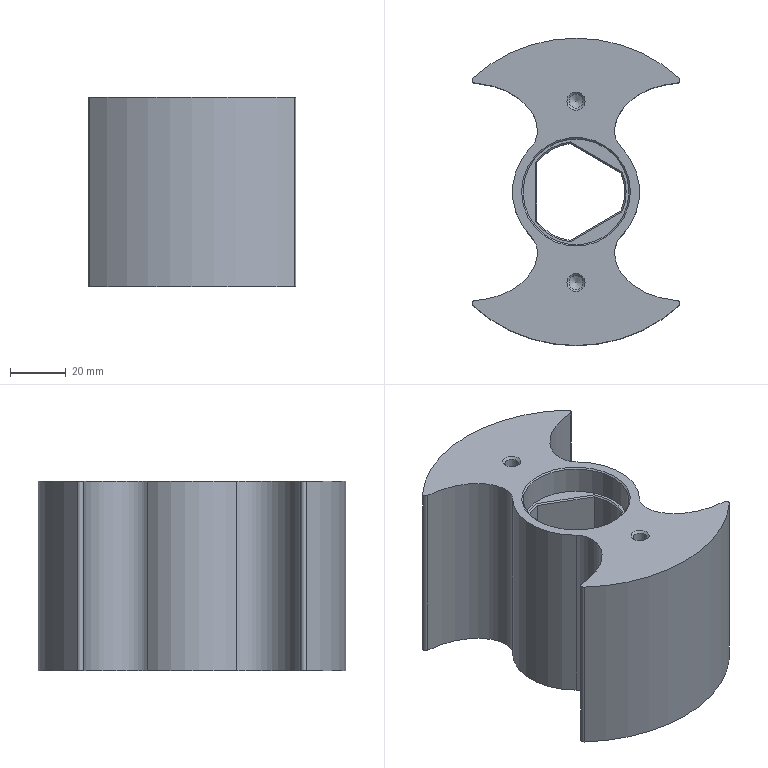NC program | NX | posted with a generic post | part box 74.46 x 110.159 x 68 mm
Lines 28 to 1004 of 5030:
(ZLEVEL_PROFILE_COPY_1 , TOOL : D12)
N48 M6
N50 G54
N52 G17 G0 G90 X7.103 Y-3.397 S3000 M3
N54 G43 Z30. H12
N56 Z-2.
N58 G94 G1 X10.893 Y3.167 Z-2.198 F1000.
N60 X10.665 Y3.958 Z-2.22
N62 X9.854 Y5.689 Z-2.27
N64 X8.765 Y7.258 Z-2.32
N66 X8.195 Y7.853 Z-2.342
N68 X8.017 Y7.85 Z-2.346
N70 X-8.183 Z-2.771
N72 X-8.282 Y7.761 Z-2.774
N74 X-8.844 Y7.163 Z-2.796
N76 X-9.887 Y5.632 Z-2.844
N78 X-10.665 Y3.951 Z-2.893
N80 X-10.89 Y3.162 Z-2.914
N82 X-2.794 Y-10.861 Z-3.338
N84 X-2.704 Y-11.023 Z-3.343
N86 X-1.898 Y-11.219 Z-3.365
N88 X-0.048 Y-11.377 Z-3.413
N90 X1.802 Y-11.235 Z-3.462
N92 X2.61 Y-11.046 Z-3.484
N94 X2.707 Y-11.012 Z-3.486
N96 X10.893 Y3.167 Z-3.915
N98 X10.665 Y3.958 Z-3.937
N100 X9.854 Y5.689 Z-3.987
N102 X8.765 Y7.258 Z-4.037
N104 X8.195 Y7.853 Z-4.058
N106 X8.017 Y7.85 Z-4.063
N108 X-8.183 Z-4.487
N110 X-8.282 Y7.761 Z-4.49
N112 X-8.844 Y7.163 Z-4.512
N114 X-9.887 Y5.632 Z-4.56
N116 X-10.665 Y3.951 Z-4.609
N118 X-10.89 Y3.162 Z-4.63
N120 X-2.794 Y-10.861 Z-5.054
N122 X-2.704 Y-11.023 Z-5.059
N124 X-1.898 Y-11.219 Z-5.081
N126 X-0.048 Y-11.377 Z-5.13
N128 X1.802 Y-11.235 Z-5.178
N130 X2.61 Y-11.046 Z-5.2
N132 X2.707 Y-11.012 F1800.
N134 X10.893 Y3.167
N136 G3 X8.195 Y7.853 R11.295
N138 G1 X8.017 Y7.85
N140 X-8.183
N142 X-8.282 Y7.761
N144 G3 X-10.89 Y3.162 R11.205
N146 G1 X-2.794 Y-10.861
N148 X-2.704 Y-11.023
N150 G3 X2.61 Y-11.046 R11.457
N152 G1 X2.691 Y-11.014 Z-5.202
N154 X3.065 Y-10.392 Z-5.214
N156 X8.385 Y-1.178 Z-5.4
N158 X10.893 Y3.167
N160 G3 X8.195 Y7.853 R11.295
N162 G1 X8.017 Y7.85
N164 X-8.183
N166 X-8.282 Y7.761
N168 G3 X-10.89 Y3.162 R11.205
N170 G1 X-2.794 Y-10.861
N172 X-2.704 Y-11.023
N174 G3 X2.61 Y-11.046 R11.457
N176 G1 X2.691 Y-11.014 Z-5.402
N178 X3.065 Y-10.392 Z-5.414
N180 X8.385 Y-1.178 Z-5.6
N182 X10.9 Y3.179
N184 X10.855 Y3.316
N186 G3 X8.195 Y7.853 R11.35
N188 G1 X8.017 Y7.85
N190 X-8.193
N192 X-8.282 Y7.761
N194 G3 X-10.859 Y3.303 R11.35
N196 G1 X-10.9 Y3.179
N198 X-2.794 Y-10.861
N200 X-2.704 Y-11.023
N202 G3 X2.61 Y-11.046 R11.35
N204 G1 X2.691 Y-11.014 Z-5.602
N206 X3.063 Y-10.394 Z-5.614
N208 X8.383 Y-1.18 Z-5.8
N210 X10.9 Y3.179
N212 X10.855 Y3.316
N214 G3 X8.195 Y7.853 R11.35
N216 G1 X8.017 Y7.85
N218 X-8.193
N220 X-8.282 Y7.761
N222 G3 X-10.859 Y3.303 R11.35
N224 G1 X-10.9 Y3.179
N226 X-2.794 Y-10.861
N228 X-2.704 Y-11.023
N230 G3 X2.61 Y-11.046 R11.35
N232 G1 X2.696 Y-11.013 Z-5.802
N234 X3.063 Y-10.394 Z-5.814
N236 X8.383 Y-1.18 Z-6.
N238 X10.9 Y3.179
N240 X10.855 Y3.316
N242 G3 X8.195 Y7.853 R11.35
N244 G1 X8.017 Y7.85
N246 X-8.193
N248 X-8.282 Y7.761
N250 G3 X-10.859 Y3.303 R11.35
N252 G1 X-10.9 Y3.179
N254 X-2.794 Y-10.861
N256 X-2.704 Y-11.023
N258 G3 X2.61 Y-11.046 R11.35
N260 G1 X2.696 Y-11.013 Z-6.002
N262 X3.063 Y-10.394 Z-6.014
N264 X8.383 Y-1.18 Z-6.2
N266 X10.9 Y3.179
N268 X10.855 Y3.316
N270 G3 X8.195 Y7.853 R11.35
N272 G1 X8.017 Y7.85
N274 X-8.193
N276 X-8.282 Y7.761
N278 G3 X-10.859 Y3.303 R11.35
N280 G1 X-10.9 Y3.179
N282 X-2.794 Y-10.861
N284 X-2.704 Y-11.023
N286 G3 X2.61 Y-11.046 R11.35
N288 G1 X2.696 Y-11.013 Z-6.202
N290 X3.063 Y-10.394 Z-6.214
N292 X8.383 Y-1.18 Z-6.4
N294 X10.9 Y3.179
N296 X10.855 Y3.316
N298 G3 X8.195 Y7.853 R11.35
N300 G1 X8.017 Y7.85
N302 X-8.193
N304 X-8.282 Y7.761
N306 G3 X-10.859 Y3.303 R11.35
N308 G1 X-10.9 Y3.179
N310 X-2.794 Y-10.861
N312 X-2.704 Y-11.023
N314 G3 X2.61 Y-11.046 R11.35
N316 G1 X2.696 Y-11.013 Z-6.402
N318 X3.063 Y-10.394 Z-6.414
N320 X8.383 Y-1.18 Z-6.6
N322 X10.9 Y3.179
N324 X10.855 Y3.316
N326 G3 X8.195 Y7.853 R11.35
N328 G1 X8.017 Y7.85
N330 X-8.193
N332 X-8.282 Y7.761
N334 G3 X-10.859 Y3.303 R11.35
N336 G1 X-10.9 Y3.179
N338 X-2.794 Y-10.861
N340 X-2.704 Y-11.023
N342 G3 X2.61 Y-11.046 R11.35
N344 G1 X2.696 Y-11.013 Z-6.602
N346 X3.063 Y-10.394 Z-6.614
N348 X8.383 Y-1.18 Z-6.8
N350 X10.9 Y3.179
N352 X10.855 Y3.316
N354 G3 X8.195 Y7.853 R11.35
N356 G1 X8.017 Y7.85
N358 X-8.193
N360 X-8.282 Y7.761
N362 G3 X-10.859 Y3.303 R11.35
N364 G1 X-10.9 Y3.179
N366 X-2.794 Y-10.861
N368 X-2.704 Y-11.023
N370 G3 X2.61 Y-11.046 R11.35
N372 G1 X2.696 Y-11.013 Z-6.802
N374 X3.063 Y-10.394 Z-6.814
N376 X8.383 Y-1.18 Z-7.
N378 X10.9 Y3.179
N380 X10.855 Y3.316
N382 G3 X8.195 Y7.853 R11.35
N384 G1 X8.017 Y7.85
N386 X-8.193
N388 X-8.282 Y7.761
N390 G3 X-10.859 Y3.303 R11.35
N392 G1 X-10.9 Y3.179
N394 X-2.794 Y-10.861
N396 X-2.704 Y-11.023
N398 G3 X2.61 Y-11.046 R11.35
N400 G1 X2.696 Y-11.013 Z-7.002
N402 X3.063 Y-10.394 Z-7.014
N404 X8.383 Y-1.18 Z-7.2
N406 X10.9 Y3.179
N408 X10.855 Y3.316
N410 G3 X8.195 Y7.853 R11.35
N412 G1 X8.017 Y7.85
N414 X-8.193
N416 X-8.282 Y7.761
N418 G3 X-10.859 Y3.303 R11.35
N420 G1 X-10.9 Y3.179
N422 X-2.794 Y-10.861
N424 X-2.704 Y-11.023
N426 G3 X2.61 Y-11.046 R11.35
N428 G1 X2.696 Y-11.013 Z-7.202
N430 X3.063 Y-10.394 Z-7.214
N432 X8.383 Y-1.18 Z-7.4
N434 X10.9 Y3.179
N436 X10.855 Y3.316
N438 G3 X8.195 Y7.853 R11.35
N440 G1 X8.017 Y7.85
N442 X-8.193
N444 X-8.282 Y7.761
N446 G3 X-10.859 Y3.303 R11.35
N448 G1 X-10.9 Y3.179
N450 X-2.794 Y-10.861
N452 X-2.704 Y-11.023
N454 G3 X2.61 Y-11.046 R11.35
N456 G1 X2.696 Y-11.013 Z-7.402
N458 X3.063 Y-10.394 Z-7.414
N460 X8.383 Y-1.18 Z-7.6
N462 X10.9 Y3.179
N464 X10.855 Y3.316
N466 G3 X8.195 Y7.853 R11.35
N468 G1 X8.017 Y7.85
N470 X-8.193
N472 X-8.282 Y7.761
N474 G3 X-10.859 Y3.303 R11.35
N476 G1 X-10.9 Y3.179
N478 X-2.794 Y-10.861
N480 X-2.704 Y-11.023
N482 G3 X2.61 Y-11.046 R11.35
N484 G1 X2.696 Y-11.013 Z-7.602
N486 X3.063 Y-10.394 Z-7.614
N488 X8.383 Y-1.18 Z-7.8
N490 X10.9 Y3.179
N492 X10.855 Y3.316
N494 G3 X8.195 Y7.853 R11.35
N496 G1 X8.017 Y7.85
N498 X-8.193
N500 X-8.282 Y7.761
N502 G3 X-10.859 Y3.303 R11.35
N504 G1 X-10.9 Y3.179
N506 X-2.794 Y-10.861
N508 X-2.704 Y-11.023
N510 G3 X2.61 Y-11.046 R11.35
N512 G1 X2.696 Y-11.013 Z-7.802
N514 X3.063 Y-10.394 Z-7.814
N516 X8.383 Y-1.18 Z-8.
N518 X10.9 Y3.179
N520 X10.855 Y3.316
N522 G3 X8.195 Y7.853 R11.35
N524 G1 X8.017 Y7.85
N526 X-8.193
N528 X-8.282 Y7.761
N530 G3 X-10.859 Y3.303 R11.35
N532 G1 X-10.9 Y3.179
N534 X-2.794 Y-10.861
N536 X-2.704 Y-11.023
N538 G3 X2.61 Y-11.046 R11.35
N540 G1 X2.696 Y-11.013 Z-8.002
N542 X3.063 Y-10.394 Z-8.014
N544 X8.383 Y-1.18 Z-8.2
N546 X10.9 Y3.179
N548 X10.855 Y3.316
N550 G3 X8.195 Y7.853 R11.35
N552 G1 X8.017 Y7.85
N554 X-8.193
N556 X-8.282 Y7.761
N558 G3 X-10.859 Y3.303 R11.35
N560 G1 X-10.9 Y3.179
N562 X-2.794 Y-10.861
N564 X-2.704 Y-11.023
N566 G3 X2.61 Y-11.046 R11.35
N568 G1 X2.696 Y-11.013 Z-8.202
N570 X3.063 Y-10.394 Z-8.214
N572 X8.383 Y-1.18 Z-8.4
N574 X10.9 Y3.179
N576 X10.855 Y3.316
N578 G3 X8.195 Y7.853 R11.35
N580 G1 X8.017 Y7.85
N582 X-8.193
N584 X-8.282 Y7.761
N586 G3 X-10.859 Y3.303 R11.35
N588 G1 X-10.9 Y3.179
N590 X-2.794 Y-10.861
N592 X-2.704 Y-11.023
N594 G3 X2.61 Y-11.046 R11.35
N596 G1 X2.696 Y-11.013 Z-8.402
N598 X3.063 Y-10.394 Z-8.414
N600 X8.383 Y-1.18 Z-8.6
N602 X10.9 Y3.179
N604 X10.855 Y3.316
N606 G3 X8.195 Y7.853 R11.35
N608 G1 X8.017 Y7.85
N610 X-8.193
N612 X-8.282 Y7.761
N614 G3 X-10.859 Y3.303 R11.35
N616 G1 X-10.9 Y3.179
N618 X-2.794 Y-10.861
N620 X-2.704 Y-11.023
N622 G3 X2.61 Y-11.046 R11.35
N624 G1 X2.696 Y-11.013 Z-8.602
N626 X3.063 Y-10.394 Z-8.614
N628 X8.383 Y-1.18 Z-8.8
N630 X10.9 Y3.179
N632 X10.855 Y3.316
N634 G3 X8.195 Y7.853 R11.35
N636 G1 X8.017 Y7.85
N638 X-8.193
N640 X-8.282 Y7.761
N642 G3 X-10.859 Y3.303 R11.35
N644 G1 X-10.9 Y3.179
N646 X-2.794 Y-10.861
N648 X-2.704 Y-11.023
N650 G3 X2.61 Y-11.046 R11.35
N652 G1 X2.696 Y-11.013 Z-8.802
N654 X3.063 Y-10.394 Z-8.814
N656 X8.383 Y-1.18 Z-9.
N658 X10.9 Y3.179
N660 X10.855 Y3.316
N662 G3 X8.195 Y7.853 R11.35
N664 G1 X8.017 Y7.85
N666 X-8.193
N668 X-8.282 Y7.761
N670 G3 X-10.859 Y3.303 R11.35
N672 G1 X-10.9 Y3.179
N674 X-2.794 Y-10.861
N676 X-2.704 Y-11.023
N678 G3 X2.61 Y-11.046 R11.35
N680 G1 X2.696 Y-11.013 Z-9.002
N682 X3.063 Y-10.394 Z-9.014
N684 X8.383 Y-1.18 Z-9.2
N686 X10.9 Y3.179
N688 X10.855 Y3.316
N690 G3 X8.195 Y7.853 R11.35
N692 G1 X8.017 Y7.85
N694 X-8.193
N696 X-8.282 Y7.761
N698 G3 X-10.859 Y3.303 R11.35
N700 G1 X-10.9 Y3.179
N702 X-2.794 Y-10.861
N704 X-2.704 Y-11.023
N706 G3 X2.61 Y-11.046 R11.35
N708 G1 X2.696 Y-11.013 Z-9.202
N710 X3.063 Y-10.394 Z-9.214
N712 X8.383 Y-1.18 Z-9.4
N714 X10.9 Y3.179
N716 X10.855 Y3.316
N718 G3 X8.195 Y7.853 R11.35
N720 G1 X8.017 Y7.85
N722 X-8.193
N724 X-8.282 Y7.761
N726 G3 X-10.859 Y3.303 R11.35
N728 G1 X-10.9 Y3.179
N730 X-2.794 Y-10.861
N732 X-2.704 Y-11.023
N734 G3 X2.61 Y-11.046 R11.35
N736 G1 X2.696 Y-11.013 Z-9.402
N738 X3.063 Y-10.394 Z-9.414
N740 X8.383 Y-1.18 Z-9.6
N742 X10.9 Y3.179
N744 X10.855 Y3.316
N746 G3 X8.195 Y7.853 R11.35
N748 G1 X8.017 Y7.85
N750 X-8.193
N752 X-8.282 Y7.761
N754 G3 X-10.859 Y3.303 R11.35
N756 G1 X-10.9 Y3.179
N758 X-2.794 Y-10.861
N760 X-2.704 Y-11.023
N762 G3 X2.61 Y-11.046 R11.35
N764 G1 X2.696 Y-11.013 Z-9.602
N766 X3.063 Y-10.394 Z-9.614
N768 X8.383 Y-1.18 Z-9.8
N770 X10.9 Y3.179
N772 X10.855 Y3.316
N774 G3 X8.195 Y7.853 R11.35
N776 G1 X8.017 Y7.85
N778 X-8.193
N780 X-8.282 Y7.761
N782 G3 X-10.859 Y3.303 R11.35
N784 G1 X-10.9 Y3.179
N786 X-2.794 Y-10.861
N788 X-2.704 Y-11.023
N790 G3 X2.61 Y-11.046 R11.35
N792 G1 X2.696 Y-11.013 Z-9.802
N794 X3.063 Y-10.394 Z-9.814
N796 X8.383 Y-1.18 Z-10.
N798 X10.9 Y3.179
N800 X10.855 Y3.316
N802 G3 X8.195 Y7.853 R11.35
N804 G1 X8.017 Y7.85
N806 X-8.193
N808 X-8.282 Y7.761
N810 G3 X-10.859 Y3.303 R11.35
N812 G1 X-10.9 Y3.179
N814 X-2.794 Y-10.861
N816 X-2.704 Y-11.023
N818 G3 X2.61 Y-11.046 R11.35
N820 G1 X2.696 Y-11.013 Z-10.002
N822 X3.063 Y-10.394 Z-10.014
N824 X8.383 Y-1.18 Z-10.2
N826 X10.9 Y3.179
N828 X10.855 Y3.316
N830 G3 X8.195 Y7.853 R11.35
N832 G1 X8.017 Y7.85
N834 X-8.193
N836 X-8.282 Y7.761
N838 G3 X-10.859 Y3.303 R11.35
N840 G1 X-10.9 Y3.179
N842 X-2.794 Y-10.861
N844 X-2.704 Y-11.023
N846 G3 X2.61 Y-11.046 R11.35
N848 G1 X2.696 Y-11.013 Z-10.202
N850 X3.063 Y-10.394 Z-10.214
N852 X8.383 Y-1.18 Z-10.4
N854 X10.9 Y3.179
N856 X10.855 Y3.316
N858 G3 X8.195 Y7.853 R11.35
N860 G1 X8.017 Y7.85
N862 X-8.193
N864 X-8.282 Y7.761
N866 G3 X-10.859 Y3.303 R11.35
N868 G1 X-10.9 Y3.179
N870 X-2.794 Y-10.861
N872 X-2.704 Y-11.023
N874 G3 X2.61 Y-11.046 R11.35
N876 G1 X2.696 Y-11.013 Z-10.402
N878 X3.063 Y-10.394 Z-10.414
N880 X8.383 Y-1.18 Z-10.6
N882 X10.9 Y3.179
N884 X10.855 Y3.316
N886 G3 X8.195 Y7.853 R11.35
N888 G1 X8.017 Y7.85
N890 X-8.193
N892 X-8.282 Y7.761
N894 G3 X-10.859 Y3.303 R11.35
N896 G1 X-10.9 Y3.179
N898 X-2.794 Y-10.861
N900 X-2.704 Y-11.023
N902 G3 X2.61 Y-11.046 R11.35
N904 G1 X2.696 Y-11.013 Z-10.602
N906 X3.063 Y-10.394 Z-10.614
N908 X8.383 Y-1.18 Z-10.8
N910 X10.9 Y3.179
N912 X10.855 Y3.316
N914 G3 X8.195 Y7.853 R11.35
N916 G1 X8.017 Y7.85
N918 X-8.193
N920 X-8.282 Y7.761
N922 G3 X-10.859 Y3.303 R11.35
N924 G1 X-10.9 Y3.179
N926 X-2.794 Y-10.861
N928 X-2.704 Y-11.023
N930 G3 X2.61 Y-11.046 R11.35
N932 G1 X2.696 Y-11.013 Z-10.802
N934 X3.063 Y-10.394 Z-10.814
N936 X8.383 Y-1.18 Z-11.
N938 X10.9 Y3.179
N940 X10.855 Y3.316
N942 G3 X8.195 Y7.853 R11.35
N944 G1 X8.017 Y7.85
N946 X-8.193
N948 X-8.282 Y7.761
N950 G3 X-10.859 Y3.303 R11.35
N952 G1 X-10.9 Y3.179
N954 X-2.794 Y-10.861
N956 X-2.704 Y-11.023
N958 G3 X2.61 Y-11.046 R11.35
N960 G1 X2.696 Y-11.013 Z-11.002
N962 X3.063 Y-10.394 Z-11.014
N964 X8.383 Y-1.18 Z-11.2
N966 X10.9 Y3.179
N968 X10.855 Y3.316
N970 G3 X8.195 Y7.853 R11.35
N972 G1 X8.017 Y7.85
N974 X-8.193
N976 X-8.282 Y7.761
N978 G3 X-10.859 Y3.303 R11.35
N980 G1 X-10.9 Y3.179
N982 X-2.794 Y-10.861
N984 X-2.704 Y-11.023
N986 G3 X2.61 Y-11.046 R11.35
N988 G1 X2.696 Y-11.013 Z-11.202
N990 X3.063 Y-10.394 Z-11.214
N992 X8.383 Y-1.18 Z-11.4
N994 X10.9 Y3.179
N996 X10.855 Y3.316
N998 G3 X8.195 Y7.853 R11.35
N1000 G1 X8.017 Y7.85
N1002 X-8.193
N1004 X-8.282 Y7.761
N1006 G3 X-10.859 Y3.303 R11.35
N1008 G1 X-10.9 Y3.179
N1010 X-2.794 Y-10.861
N1012 X-2.704 Y-11.023
N1014 G3 X2.61 Y-11.046 R11.35
N1016 G1 X2.696 Y-11.013 Z-11.402
N1018 X3.063 Y-10.394 Z-11.414
N1020 X8.383 Y-1.18 Z-11.6
N1022 X10.9 Y3.179
N1024 X10.855 Y3.316
N1026 G3 X8.195 Y7.853 R11.35
N1028 G1 X8.017 Y7.85
N1030 X-8.193
N1032 X-8.282 Y7.761
N1034 G3 X-10.859 Y3.303 R11.35
N1036 G1 X-10.9 Y3.179
N1038 X-2.794 Y-10.861
N1040 X-2.704 Y-11.023
N1042 G3 X2.61 Y-11.046 R11.35
N1044 G1 X2.696 Y-11.013 Z-11.602
N1046 X3.063 Y-10.394 Z-11.614
N1048 X8.383 Y-1.18 Z-11.8
N1050 X10.9 Y3.179
N1052 X10.855 Y3.316
N1054 G3 X8.195 Y7.853 R11.35
N1056 G1 X8.017 Y7.85
N1058 X-8.193
N1060 X-8.282 Y7.761
N1062 G3 X-10.859 Y3.303 R11.35
N1064 G1 X-10.9 Y3.179
N1066 X-2.794 Y-10.861
N1068 X-2.704 Y-11.023
N1070 G3 X2.61 Y-11.046 R11.35
N1072 G1 X2.696 Y-11.013 Z-11.802
N1074 X3.063 Y-10.394 Z-11.814
N1076 X8.383 Y-1.18 Z-12.
N1078 X10.9 Y3.179
N1080 X10.855 Y3.316
N1082 G3 X8.195 Y7.853 R11.35
N1084 G1 X8.017 Y7.85
N1086 X-8.193
N1088 X-8.282 Y7.761
N1090 G3 X-10.859 Y3.303 R11.35
N1092 G1 X-10.9 Y3.179
N1094 X-2.794 Y-10.861
N1096 X-2.704 Y-11.023
N1098 G3 X2.61 Y-11.046 R11.35
N1100 G1 X2.696 Y-11.013 Z-12.002
N1102 X3.063 Y-10.394 Z-12.014
N1104 X8.383 Y-1.18 Z-12.2
N1106 X10.9 Y3.179
N1108 X10.855 Y3.316
N1110 G3 X8.195 Y7.853 R11.35
N1112 G1 X8.017 Y7.85
N1114 X-8.193
N1116 X-8.282 Y7.761
N1118 G3 X-10.859 Y3.303 R11.35
N1120 G1 X-10.9 Y3.179
N1122 X-2.794 Y-10.861
N1124 X-2.704 Y-11.023
N1126 G3 X2.61 Y-11.046 R11.35
N1128 G1 X2.696 Y-11.013 Z-12.202
N1130 X3.063 Y-10.394 Z-12.214
N1132 X8.383 Y-1.18 Z-12.4
N1134 X10.9 Y3.179
N1136 X10.855 Y3.316
N1138 G3 X8.195 Y7.853 R11.35
N1140 G1 X8.017 Y7.85
N1142 X-8.193
N1144 X-8.282 Y7.761
N1146 G3 X-10.859 Y3.303 R11.35
N1148 G1 X-10.9 Y3.179
N1150 X-2.794 Y-10.861
N1152 X-2.704 Y-11.023
N1154 G3 X2.61 Y-11.046 R11.35
N1156 G1 X2.696 Y-11.013 Z-12.402
N1158 X3.063 Y-10.394 Z-12.414
N1160 X8.383 Y-1.18 Z-12.6
N1162 X10.9 Y3.179
N1164 X10.855 Y3.316
N1166 G3 X8.195 Y7.853 R11.35
N1168 G1 X8.017 Y7.85
N1170 X-8.193
N1172 X-8.282 Y7.761
N1174 G3 X-10.859 Y3.303 R11.35
N1176 G1 X-10.9 Y3.179
N1178 X-2.794 Y-10.861
N1180 X-2.704 Y-11.023
N1182 G3 X2.61 Y-11.046 R11.35
N1184 G1 X2.696 Y-11.013 Z-12.602
N1186 X3.063 Y-10.394 Z-12.614
N1188 X8.383 Y-1.18 Z-12.8
N1190 X10.9 Y3.179
N1192 X10.855 Y3.316
N1194 G3 X8.195 Y7.853 R11.35
N1196 G1 X8.017 Y7.85
N1198 X-8.193
N1200 X-8.282 Y7.761
N1202 G3 X-10.859 Y3.303 R11.35
N1204 G1 X-10.9 Y3.179
N1206 X-2.794 Y-10.861
N1208 X-2.704 Y-11.023
N1210 G3 X2.61 Y-11.046 R11.35
N1212 G1 X2.696 Y-11.013 Z-12.802
N1214 X3.063 Y-10.394 Z-12.814
N1216 X8.383 Y-1.18 Z-13.
N1218 X10.9 Y3.179
N1220 X10.855 Y3.316
N1222 G3 X8.195 Y7.853 R11.35
N1224 G1 X8.017 Y7.85
N1226 X-8.193
N1228 X-8.282 Y7.761
N1230 G3 X-10.859 Y3.303 R11.35
N1232 G1 X-10.9 Y3.179
N1234 X-2.794 Y-10.861
N1236 X-2.704 Y-11.023
N1238 G3 X2.61 Y-11.046 R11.35
N1240 G1 X2.696 Y-11.013 Z-13.002
N1242 X3.063 Y-10.394 Z-13.014
N1244 X8.383 Y-1.18 Z-13.2
N1246 X10.9 Y3.179
N1248 X10.855 Y3.316
N1250 G3 X8.195 Y7.853 R11.35
N1252 G1 X8.017 Y7.85
N1254 X-8.193
N1256 X-8.282 Y7.761
N1258 G3 X-10.859 Y3.303 R11.35
N1260 G1 X-10.9 Y3.179
N1262 X-2.794 Y-10.861
N1264 X-2.704 Y-11.023
N1266 G3 X2.61 Y-11.046 R11.35
N1268 G1 X2.696 Y-11.013 Z-13.202
N1270 X3.063 Y-10.394 Z-13.214
N1272 X8.383 Y-1.18 Z-13.4
N1274 X10.9 Y3.179
N1276 X10.855 Y3.316
N1278 G3 X8.195 Y7.853 R11.35
N1280 G1 X8.017 Y7.85
N1282 X-8.193
N1284 X-8.282 Y7.761
N1286 G3 X-10.859 Y3.303 R11.35
N1288 G1 X-10.9 Y3.179
N1290 X-2.794 Y-10.861
N1292 X-2.704 Y-11.023
N1294 G3 X2.61 Y-11.046 R11.35
N1296 G1 X2.696 Y-11.013 Z-13.402
N1298 X3.063 Y-10.394 Z-13.414
N1300 X8.383 Y-1.18 Z-13.6
N1302 X10.9 Y3.179
N1304 X10.855 Y3.316
N1306 G3 X8.195 Y7.853 R11.35
N1308 G1 X8.017 Y7.85
N1310 X-8.193
N1312 X-8.282 Y7.761
N1314 G3 X-10.859 Y3.303 R11.35
N1316 G1 X-10.9 Y3.179
N1318 X-2.794 Y-10.861
N1320 X-2.704 Y-11.023
N1322 G3 X2.61 Y-11.046 R11.35
N1324 G1 X2.696 Y-11.013 Z-13.602
N1326 X3.063 Y-10.394 Z-13.614
N1328 X8.383 Y-1.18 Z-13.8
N1330 X10.9 Y3.179
N1332 X10.855 Y3.316
N1334 G3 X8.195 Y7.853 R11.35
N1336 G1 X8.017 Y7.85
N1338 X-8.193
N1340 X-8.282 Y7.761
N1342 G3 X-10.859 Y3.303 R11.35
N1344 G1 X-10.9 Y3.179
N1346 X-2.794 Y-10.861
N1348 X-2.704 Y-11.023
N1350 G3 X2.61 Y-11.046 R11.35
N1352 G1 X2.696 Y-11.013 Z-13.802
N1354 X3.063 Y-10.394 Z-13.814
N1356 X8.383 Y-1.18 Z-14.
N1358 X10.9 Y3.179
N1360 X10.855 Y3.316
N1362 G3 X8.195 Y7.853 R11.35
N1364 G1 X8.017 Y7.85
N1366 X-8.193
N1368 X-8.282 Y7.761
N1370 G3 X-10.859 Y3.303 R11.35
N1372 G1 X-10.9 Y3.179
N1374 X-2.794 Y-10.861
N1376 X-2.704 Y-11.023
N1378 G3 X2.61 Y-11.046 R11.35
N1380 G1 X2.696 Y-11.013 Z-14.002
N1382 X3.063 Y-10.394 Z-14.014
N1384 X8.383 Y-1.18 Z-14.2
N1386 X10.9 Y3.179
N1388 X10.855 Y3.316
N1390 G3 X8.195 Y7.853 R11.35
N1392 G1 X8.017 Y7.85
N1394 X-8.193
N1396 X-8.282 Y7.761
N1398 G3 X-10.859 Y3.303 R11.35
N1400 G1 X-10.9 Y3.179
N1402 X-2.794 Y-10.861
N1404 X-2.704 Y-11.023
N1406 G3 X2.61 Y-11.046 R11.35
N1408 G1 X2.696 Y-11.013 Z-14.202
N1410 X3.063 Y-10.394 Z-14.214
N1412 X8.383 Y-1.18 Z-14.4
N1414 X10.9 Y3.179
N1416 X10.855 Y3.316
N1418 G3 X8.195 Y7.853 R11.35
N1420 G1 X8.017 Y7.85
N1422 X-8.193
N1424 X-8.282 Y7.761
N1426 G3 X-10.859 Y3.303 R11.35
N1428 G1 X-10.9 Y3.179
N1430 X-2.794 Y-10.861
N1432 X-2.704 Y-11.023
N1434 G3 X2.61 Y-11.046 R11.35
N1436 G1 X2.696 Y-11.013 Z-14.402
N1438 X3.063 Y-10.394 Z-14.414
N1440 X8.383 Y-1.18 Z-14.6
N1442 X10.9 Y3.179
N1444 X10.855 Y3.316
N1446 G3 X8.195 Y7.853 R11.35
N1448 G1 X8.017 Y7.85
N1450 X-8.193
N1452 X-8.282 Y7.761
N1454 G3 X-10.859 Y3.303 R11.35
N1456 G1 X-10.9 Y3.179
N1458 X-2.794 Y-10.861
N1460 X-2.704 Y-11.023
N1462 G3 X2.61 Y-11.046 R11.35
N1464 G1 X2.696 Y-11.013 Z-14.602
N1466 X3.063 Y-10.394 Z-14.614
N1468 X8.383 Y-1.18 Z-14.8
N1470 X10.9 Y3.179
N1472 X10.855 Y3.316
N1474 G3 X8.195 Y7.853 R11.35
N1476 G1 X8.017 Y7.85
N1478 X-8.193
N1480 X-8.282 Y7.761
N1482 G3 X-10.859 Y3.303 R11.35
N1484 G1 X-10.9 Y3.179
N1486 X-2.794 Y-10.861
N1488 X-2.704 Y-11.023
N1490 G3 X2.61 Y-11.046 R11.35
N1492 G1 X2.696 Y-11.013 Z-14.802
N1494 X3.063 Y-10.394 Z-14.814
N1496 X8.383 Y-1.18 Z-15.
N1498 X10.9 Y3.179
N1500 X10.855 Y3.316
N1502 G3 X8.195 Y7.853 R11.35
N1504 G1 X8.017 Y7.85
N1506 X-8.193
N1508 X-8.282 Y7.761
N1510 G3 X-10.859 Y3.303 R11.35
N1512 G1 X-10.9 Y3.179
N1514 X-2.794 Y-10.861
N1516 X-2.704 Y-11.023
N1518 G3 X2.61 Y-11.046 R11.35
N1520 G1 X2.696 Y-11.013 Z-15.002
N1522 X3.063 Y-10.394 Z-15.014
N1524 X8.383 Y-1.18 Z-15.2
N1526 X10.9 Y3.179
N1528 X10.855 Y3.316
N1530 G3 X8.195 Y7.853 R11.35
N1532 G1 X8.017 Y7.85
N1534 X-8.193
N1536 X-8.282 Y7.761
N1538 G3 X-10.859 Y3.303 R11.35
N1540 G1 X-10.9 Y3.179
N1542 X-2.794 Y-10.861
N1544 X-2.704 Y-11.023
N1546 G3 X2.61 Y-11.046 R11.35
N1548 G1 X2.696 Y-11.013 Z-15.202
N1550 X3.063 Y-10.394 Z-15.214
N1552 X8.383 Y-1.18 Z-15.4
N1554 X10.9 Y3.179
N1556 X10.855 Y3.316
N1558 G3 X8.195 Y7.853 R11.35
N1560 G1 X8.017 Y7.85
N1562 X-8.193
N1564 X-8.282 Y7.761
N1566 G3 X-10.859 Y3.303 R11.35
N1568 G1 X-10.9 Y3.179
N1570 X-2.794 Y-10.861
N1572 X-2.704 Y-11.023
N1574 G3 X2.61 Y-11.046 R11.35
N1576 G1 X2.696 Y-11.013 Z-15.402
N1578 X3.063 Y-10.394 Z-15.414
N1580 X8.383 Y-1.18 Z-15.6
N1582 X10.9 Y3.179
N1584 X10.855 Y3.316
N1586 G3 X8.195 Y7.853 R11.35
N1588 G1 X8.017 Y7.85
N1590 X-8.193
N1592 X-8.282 Y7.761
N1594 G3 X-10.859 Y3.303 R11.35
N1596 G1 X-10.9 Y3.179
N1598 X-2.794 Y-10.861
N1600 X-2.704 Y-11.023
N1602 G3 X2.61 Y-11.046 R11.35
N1604 G1 X2.696 Y-11.013 Z-15.602
N1606 X3.063 Y-10.394 Z-15.614
N1608 X8.383 Y-1.18 Z-15.8
N1610 X10.9 Y3.179
N1612 X10.855 Y3.316
N1614 G3 X8.195 Y7.853 R11.35
N1616 G1 X8.017 Y7.85
N1618 X-8.193
N1620 X-8.282 Y7.761
N1622 G3 X-10.859 Y3.303 R11.35
N1624 G1 X-10.9 Y3.179
N1626 X-2.794 Y-10.861
N1628 X-2.704 Y-11.023
N1630 G3 X2.61 Y-11.046 R11.35
N1632 G1 X2.696 Y-11.013 Z-15.802
N1634 X3.063 Y-10.394 Z-15.814
N1636 X8.383 Y-1.18 Z-16.
N1638 X10.9 Y3.179
N1640 X10.855 Y3.316
N1642 G3 X8.195 Y7.853 R11.35
N1644 G1 X8.017 Y7.85
N1646 X-8.193
N1648 X-8.282 Y7.761
N1650 G3 X-10.859 Y3.303 R11.35
N1652 G1 X-10.9 Y3.179
N1654 X-2.794 Y-10.861
N1656 X-2.704 Y-11.023
N1658 G3 X2.61 Y-11.046 R11.35
N1660 G1 X2.696 Y-11.013 Z-16.002
N1662 X3.063 Y-10.394 Z-16.014
N1664 X8.383 Y-1.18 Z-16.2
N1666 X10.9 Y3.179
N1668 X10.855 Y3.316
N1670 G3 X8.195 Y7.853 R11.35
N1672 G1 X8.017 Y7.85
N1674 X-8.193
N1676 X-8.282 Y7.761
N1678 G3 X-10.859 Y3.303 R11.35
N1680 G1 X-10.9 Y3.179
N1682 X-2.794 Y-10.861
N1684 X-2.704 Y-11.023
N1686 G3 X2.61 Y-11.046 R11.35
N1688 G1 X2.696 Y-11.013 Z-16.202
N1690 X3.063 Y-10.394 Z-16.214
N1692 X8.383 Y-1.18 Z-16.4
N1694 X10.9 Y3.179
N1696 X10.855 Y3.316
N1698 G3 X8.195 Y7.853 R11.35
N1700 G1 X8.017 Y7.85
N1702 X-8.193
N1704 X-8.282 Y7.761
N1706 G3 X-10.859 Y3.303 R11.35
N1708 G1 X-10.9 Y3.179
N1710 X-2.794 Y-10.861
N1712 X-2.704 Y-11.023
N1714 G3 X2.61 Y-11.046 R11.35
N1716 G1 X2.696 Y-11.013 Z-16.402
N1718 X3.063 Y-10.394 Z-16.414
N1720 X8.383 Y-1.18 Z-16.6
N1722 X10.9 Y3.179
N1724 X10.855 Y3.316
N1726 G3 X8.195 Y7.853 R11.35
N1728 G1 X8.017 Y7.85
N1730 X-8.193
N1732 X-8.282 Y7.761
N1734 G3 X-10.859 Y3.303 R11.35
N1736 G1 X-10.9 Y3.179
N1738 X-2.794 Y-10.861
N1740 X-2.704 Y-11.023
N1742 G3 X2.61 Y-11.046 R11.35
N1744 G1 X2.696 Y-11.013 Z-16.602
N1746 X3.063 Y-10.394 Z-16.614
N1748 X8.383 Y-1.18 Z-16.8
N1750 X10.9 Y3.179
N1752 X10.855 Y3.316
N1754 G3 X8.195 Y7.853 R11.35
N1756 G1 X8.017 Y7.85
N1758 X-8.193
N1760 X-8.282 Y7.761
N1762 G3 X-10.859 Y3.303 R11.35
N1764 G1 X-10.9 Y3.179
N1766 X-2.794 Y-10.861
N1768 X-2.704 Y-11.023
N1770 G3 X2.61 Y-11.046 R11.35
N1772 G1 X2.696 Y-11.013 Z-16.802
N1774 X3.063 Y-10.394 Z-16.814
N1776 X8.383 Y-1.18 Z-17.
N1778 X10.9 Y3.179
N1780 X10.855 Y3.316
N1782 G3 X8.195 Y7.853 R11.35
N1784 G1 X8.017 Y7.85
N1786 X-8.193
N1788 X-8.282 Y7.761
N1790 G3 X-10.859 Y3.303 R11.35
N1792 G1 X-10.9 Y3.179
N1794 X-2.794 Y-10.861
N1796 X-2.704 Y-11.023
N1798 G3 X2.61 Y-11.046 R11.35
N1800 G1 X2.696 Y-11.013 Z-17.002
N1802 X3.063 Y-10.394 Z-17.014
N1804 X8.383 Y-1.18 Z-17.2
N1806 X10.9 Y3.179
N1808 X10.855 Y3.316
N1810 G3 X8.195 Y7.853 R11.35
N1812 G1 X8.017 Y7.85
N1814 X-8.193
N1816 X-8.282 Y7.761
N1818 G3 X-10.859 Y3.303 R11.35
N1820 G1 X-10.9 Y3.179
N1822 X-2.794 Y-10.861
N1824 X-2.704 Y-11.023
N1826 G3 X2.61 Y-11.046 R11.35
N1828 G1 X2.696 Y-11.013 Z-17.202
N1830 X3.063 Y-10.394 Z-17.214
N1832 X8.383 Y-1.18 Z-17.4
N1834 X10.9 Y3.179
N1836 X10.855 Y3.316
N1838 G3 X8.195 Y7.853 R11.35
N1840 G1 X8.017 Y7.85
N1842 X-8.193
N1844 X-8.282 Y7.761
N1846 G3 X-10.859 Y3.303 R11.35
N1848 G1 X-10.9 Y3.179
N1850 X-2.794 Y-10.861
N1852 X-2.704 Y-11.023
N1854 G3 X2.61 Y-11.046 R11.35
N1856 G1 X2.696 Y-11.013 Z-17.402
N1858 X3.063 Y-10.394 Z-17.414
N1860 X8.383 Y-1.18 Z-17.6
N1862 X10.9 Y3.179
N1864 X10.855 Y3.316
N1866 G3 X8.195 Y7.853 R11.35
N1868 G1 X8.017 Y7.85
N1870 X-8.193
N1872 X-8.282 Y7.761
N1874 G3 X-10.859 Y3.303 R11.35
N1876 G1 X-10.9 Y3.179
N1878 X-2.794 Y-10.861
N1880 X-2.704 Y-11.023
N1882 G3 X2.61 Y-11.046 R11.35
N1884 G1 X2.696 Y-11.013 Z-17.602
N1886 X3.063 Y-10.394 Z-17.614
N1888 X8.383 Y-1.18 Z-17.8
N1890 X10.9 Y3.179
N1892 X10.855 Y3.316
N1894 G3 X8.195 Y7.853 R11.35
N1896 G1 X8.017 Y7.85
N1898 X-8.193
N1900 X-8.282 Y7.761
N1902 G3 X-10.859 Y3.303 R11.35
N1904 G1 X-10.9 Y3.179
N1906 X-2.794 Y-10.861
N1908 X-2.704 Y-11.023
N1910 G3 X2.61 Y-11.046 R11.35
N1912 G1 X2.696 Y-11.013 Z-17.802
N1914 X3.063 Y-10.394 Z-17.814
N1916 X8.383 Y-1.18 Z-18.
N1918 X10.9 Y3.179
N1920 X10.855 Y3.316
N1922 G3 X8.195 Y7.853 R11.35
N1924 G1 X8.017 Y7.85
N1926 X-8.193
N1928 X-8.282 Y7.761
N1930 G3 X-10.859 Y3.303 R11.35
N1932 G1 X-10.9 Y3.179
N1934 X-2.794 Y-10.861
N1936 X-2.704 Y-11.023
N1938 G3 X2.61 Y-11.046 R11.35
N1940 G1 X2.696 Y-11.013 Z-18.002
N1942 X3.063 Y-10.394 Z-18.014
N1944 X8.383 Y-1.18 Z-18.2
N1946 X10.9 Y3.179
N1948 X10.855 Y3.316
N1950 G3 X8.195 Y7.853 R11.35
N1952 G1 X8.017 Y7.85
N1954 X-8.193
N1956 X-8.282 Y7.761
N1958 G3 X-10.859 Y3.303 R11.35
N1960 G1 X-10.9 Y3.179
N1962 X-2.794 Y-10.861
N1964 X-2.704 Y-11.023
N1966 G3 X2.61 Y-11.046 R11.35
N1968 G1 X2.696 Y-11.013 Z-18.202
N1970 X3.063 Y-10.394 Z-18.214
N1972 X8.383 Y-1.18 Z-18.4
N1974 X10.9 Y3.179
N1976 X10.855 Y3.316
N1978 G3 X8.195 Y7.853 R11.35
N1980 G1 X8.017 Y7.85
N1982 X-8.193
N1984 X-8.282 Y7.761
N1986 G3 X-10.859 Y3.303 R11.35
N1988 G1 X-10.9 Y3.179
N1990 X-2.794 Y-10.861
N1992 X-2.704 Y-11.023
N1994 G3 X2.61 Y-11.046 R11.35